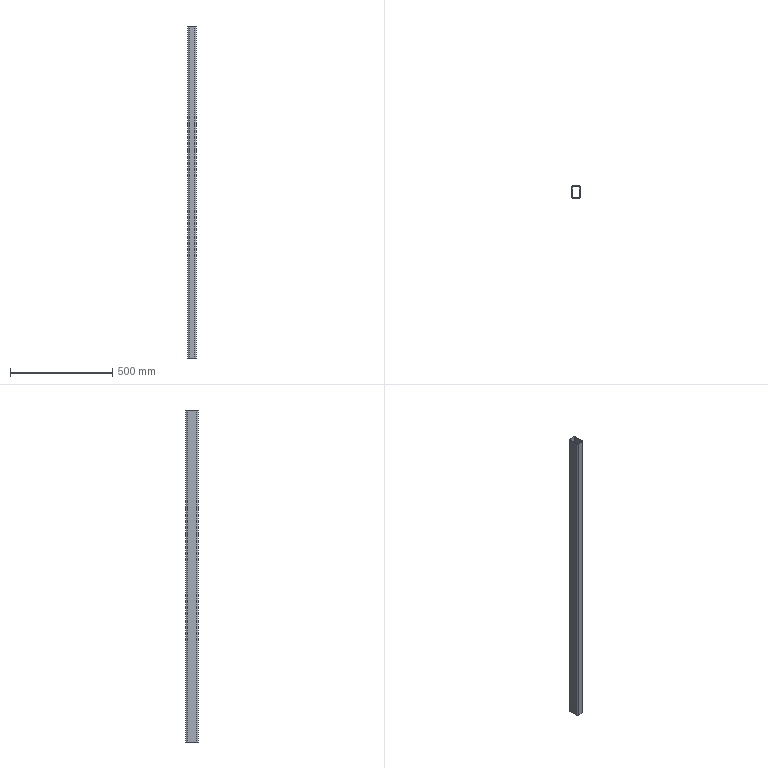Part | STEP file | Profile 40601620 | 1 solid | 18 faces | box 40 x 60 x 1620 mm | volume 927725 mm3 | plane 10 | cylinder 8 | commonest cylinder face diameters 6.4 x4 12.8 x4
STEP:
#1=CARTESIAN_POINT('',(0.,53.6,1020.));
#2=VERTEX_POINT('',#1);
#3=CARTESIAN_POINT('',(0.,6.4,1020.));
#4=VERTEX_POINT('',#3);
#5=CARTESIAN_POINT('',(0.,6.4,1020.));
#6=DIRECTION('',(0.,-1.,0.));
#7=VECTOR('',#6,1000.);
#8=LINE('',#5,#7);
#9=EDGE_CURVE('',#2,#4,#8,.T.);
#10=ORIENTED_EDGE('',*,*,#9,.F.);
#11=CARTESIAN_POINT('',(0.,53.6,-600.));
#12=VERTEX_POINT('',#11);
#13=CARTESIAN_POINT('',(0.,53.6,600.));
#14=DIRECTION('',(0.,0.,1.));
#15=VECTOR('',#14,1000.);
#16=LINE('',#13,#15);
#17=EDGE_CURVE('',#12,#2,#16,.T.);
#18=ORIENTED_EDGE('',*,*,#17,.F.);
#19=CARTESIAN_POINT('',(0.,6.4,-600.));
#20=VERTEX_POINT('',#19);
#21=CARTESIAN_POINT('',(0.,6.4,-600.));
#22=DIRECTION('',(0.,1.,0.));
#23=VECTOR('',#22,1000.);
#24=LINE('',#21,#23);
#25=EDGE_CURVE('',#20,#12,#24,.T.);
#26=ORIENTED_EDGE('',*,*,#25,.F.);
#27=CARTESIAN_POINT('',(0.,6.4,600.));
#28=DIRECTION('',(0.,0.,-1.));
#29=VECTOR('',#28,1000.);
#30=LINE('',#27,#29);
#31=EDGE_CURVE('',#4,#20,#30,.T.);
#32=ORIENTED_EDGE('',*,*,#31,.F.);
#33=EDGE_LOOP('',(#10,#18,#26,#32));
#34=FACE_OUTER_BOUND('',#33,.T.);
#35=CARTESIAN_POINT('',(0.,6.4,600.));
#36=DIRECTION('',(1.,0.,0.));
#37=DIRECTION('',(0.,1.,0.));
#38=AXIS2_PLACEMENT_3D('',#35,#36,#37);
#39=PLANE('',#38);
#40=ADVANCED_FACE('',(#34),#39,.F.);
#41=ORIENTED_EDGE('',*,*,#31,.T.);
#42=CARTESIAN_POINT('',(6.4,0.,-600.));
#43=VERTEX_POINT('',#42);
#44=CARTESIAN_POINT('',(6.4,6.4,-600.));
#45=DIRECTION('',(0.,0.,1.));
#46=DIRECTION('',(-1.,0.,0.));
#47=AXIS2_PLACEMENT_3D('',#44,#45,#46);
#48=CIRCLE('',#47,6.4);
#49=EDGE_CURVE('',#20,#43,#48,.T.);
#50=ORIENTED_EDGE('',*,*,#49,.T.);
#51=CARTESIAN_POINT('',(6.4,0.,1020.));
#52=VERTEX_POINT('',#51);
#53=CARTESIAN_POINT('',(6.4,0.,600.));
#54=DIRECTION('',(0.,0.,1.));
#55=VECTOR('',#54,1000.);
#56=LINE('',#53,#55);
#57=EDGE_CURVE('',#43,#52,#56,.T.);
#58=ORIENTED_EDGE('',*,*,#57,.T.);
#59=CARTESIAN_POINT('',(6.4,6.4,1020.));
#60=DIRECTION('',(0.,0.,-1.));
#61=DIRECTION('',(-1.,0.,0.));
#62=AXIS2_PLACEMENT_3D('',#59,#60,#61);
#63=CIRCLE('',#62,6.4);
#64=EDGE_CURVE('',#52,#4,#63,.T.);
#65=ORIENTED_EDGE('',*,*,#64,.T.);
#66=EDGE_LOOP('',(#41,#50,#58,#65));
#67=FACE_OUTER_BOUND('',#66,.T.);
#68=CARTESIAN_POINT('',(6.4,6.4,600.));
#69=DIRECTION('',(0.,0.,-1.));
#70=DIRECTION('',(-1.,0.,0.));
#71=AXIS2_PLACEMENT_3D('',#68,#69,#70);
#72=CYLINDRICAL_SURFACE('',#71,6.4);
#73=ADVANCED_FACE('',(#67),#72,.T.);
#74=CARTESIAN_POINT('',(6.4,56.8,1020.));
#75=VERTEX_POINT('',#74);
#76=CARTESIAN_POINT('',(33.6,56.8,1020.));
#77=VERTEX_POINT('',#76);
#78=CARTESIAN_POINT('',(33.6,56.8,1020.));
#79=DIRECTION('',(1.,0.,0.));
#80=VECTOR('',#79,1000.);
#81=LINE('',#78,#80);
#82=EDGE_CURVE('',#75,#77,#81,.T.);
#83=ORIENTED_EDGE('',*,*,#82,.T.);
#84=CARTESIAN_POINT('',(36.8,53.6,1020.));
#85=VERTEX_POINT('',#84);
#86=CARTESIAN_POINT('',(33.6,53.6,1020.));
#87=DIRECTION('',(0.,0.,-1.));
#88=DIRECTION('',(-1.,0.,0.));
#89=AXIS2_PLACEMENT_3D('',#86,#87,#88);
#90=CIRCLE('',#89,3.2);
#91=EDGE_CURVE('',#77,#85,#90,.T.);
#92=ORIENTED_EDGE('',*,*,#91,.T.);
#93=CARTESIAN_POINT('',(36.8,6.4,1020.));
#94=VERTEX_POINT('',#93);
#95=CARTESIAN_POINT('',(36.8,6.4,1020.));
#96=DIRECTION('',(0.,-1.,0.));
#97=VECTOR('',#96,1000.);
#98=LINE('',#95,#97);
#99=EDGE_CURVE('',#85,#94,#98,.T.);
#100=ORIENTED_EDGE('',*,*,#99,.T.);
#101=CARTESIAN_POINT('',(33.6,3.2,1020.));
#102=VERTEX_POINT('',#101);
#103=CARTESIAN_POINT('',(33.6,6.4,1020.));
#104=DIRECTION('',(0.,0.,-1.));
#105=DIRECTION('',(-1.,0.,0.));
#106=AXIS2_PLACEMENT_3D('',#103,#104,#105);
#107=CIRCLE('',#106,3.2);
#108=EDGE_CURVE('',#94,#102,#107,.T.);
#109=ORIENTED_EDGE('',*,*,#108,.T.);
#110=CARTESIAN_POINT('',(6.4,3.2,1020.));
#111=VERTEX_POINT('',#110);
#112=CARTESIAN_POINT('',(33.6,3.2,1020.));
#113=DIRECTION('',(-1.,0.,0.));
#114=VECTOR('',#113,1000.);
#115=LINE('',#112,#114);
#116=EDGE_CURVE('',#102,#111,#115,.T.);
#117=ORIENTED_EDGE('',*,*,#116,.T.);
#118=CARTESIAN_POINT('',(3.2,6.4,1020.));
#119=VERTEX_POINT('',#118);
#120=CARTESIAN_POINT('',(6.4,6.4,1020.));
#121=DIRECTION('',(0.,0.,-1.));
#122=DIRECTION('',(-1.,0.,0.));
#123=AXIS2_PLACEMENT_3D('',#120,#121,#122);
#124=CIRCLE('',#123,3.2);
#125=EDGE_CURVE('',#111,#119,#124,.T.);
#126=ORIENTED_EDGE('',*,*,#125,.T.);
#127=CARTESIAN_POINT('',(3.2,53.6,1020.));
#128=VERTEX_POINT('',#127);
#129=CARTESIAN_POINT('',(3.2,6.4,1020.));
#130=DIRECTION('',(0.,1.,0.));
#131=VECTOR('',#130,1000.);
#132=LINE('',#129,#131);
#133=EDGE_CURVE('',#119,#128,#132,.T.);
#134=ORIENTED_EDGE('',*,*,#133,.T.);
#135=CARTESIAN_POINT('',(6.4,53.6,1020.));
#136=DIRECTION('',(0.,0.,-1.));
#137=DIRECTION('',(-1.,0.,0.));
#138=AXIS2_PLACEMENT_3D('',#135,#136,#137);
#139=CIRCLE('',#138,3.2);
#140=EDGE_CURVE('',#128,#75,#139,.T.);
#141=ORIENTED_EDGE('',*,*,#140,.T.);
#142=EDGE_LOOP('',(#83,#92,#100,#109,#117,#126,#134,#141));
#143=FACE_BOUND('',#142,.T.);
#144=ORIENTED_EDGE('',*,*,#64,.F.);
#145=CARTESIAN_POINT('',(33.6,0.,1020.));
#146=VERTEX_POINT('',#145);
#147=CARTESIAN_POINT('',(33.6,0.,1020.));
#148=DIRECTION('',(1.,0.,0.));
#149=VECTOR('',#148,1000.);
#150=LINE('',#147,#149);
#151=EDGE_CURVE('',#52,#146,#150,.T.);
#152=ORIENTED_EDGE('',*,*,#151,.T.);
#153=CARTESIAN_POINT('',(40.,6.4,1020.));
#154=VERTEX_POINT('',#153);
#155=CARTESIAN_POINT('',(33.6,6.4,1020.));
#156=DIRECTION('',(0.,0.,1.));
#157=DIRECTION('',(-1.,0.,0.));
#158=AXIS2_PLACEMENT_3D('',#155,#156,#157);
#159=CIRCLE('',#158,6.4);
#160=EDGE_CURVE('',#146,#154,#159,.T.);
#161=ORIENTED_EDGE('',*,*,#160,.T.);
#162=CARTESIAN_POINT('',(40.,53.6,1020.));
#163=VERTEX_POINT('',#162);
#164=CARTESIAN_POINT('',(40.,6.4,1020.));
#165=DIRECTION('',(0.,1.,0.));
#166=VECTOR('',#165,1000.);
#167=LINE('',#164,#166);
#168=EDGE_CURVE('',#154,#163,#167,.T.);
#169=ORIENTED_EDGE('',*,*,#168,.T.);
#170=CARTESIAN_POINT('',(33.6,60.,1020.));
#171=VERTEX_POINT('',#170);
#172=CARTESIAN_POINT('',(33.6,53.6,1020.));
#173=DIRECTION('',(0.,0.,1.));
#174=DIRECTION('',(-1.,0.,0.));
#175=AXIS2_PLACEMENT_3D('',#172,#173,#174);
#176=CIRCLE('',#175,6.4);
#177=EDGE_CURVE('',#163,#171,#176,.T.);
#178=ORIENTED_EDGE('',*,*,#177,.T.);
#179=CARTESIAN_POINT('',(6.4,60.,1020.));
#180=VERTEX_POINT('',#179);
#181=CARTESIAN_POINT('',(33.6,60.,1020.));
#182=DIRECTION('',(-1.,0.,0.));
#183=VECTOR('',#182,1000.);
#184=LINE('',#181,#183);
#185=EDGE_CURVE('',#171,#180,#184,.T.);
#186=ORIENTED_EDGE('',*,*,#185,.T.);
#187=CARTESIAN_POINT('',(6.4,53.6,1020.));
#188=DIRECTION('',(0.,0.,1.));
#189=DIRECTION('',(-1.,0.,0.));
#190=AXIS2_PLACEMENT_3D('',#187,#188,#189);
#191=CIRCLE('',#190,6.4);
#192=EDGE_CURVE('',#180,#2,#191,.T.);
#193=ORIENTED_EDGE('',*,*,#192,.T.);
#194=ORIENTED_EDGE('',*,*,#9,.T.);
#195=EDGE_LOOP('',(#144,#152,#161,#169,#178,#186,#193,#194));
#196=FACE_OUTER_BOUND('',#195,.T.);
#197=CARTESIAN_POINT('',(33.6,6.4,1020.));
#198=DIRECTION('',(0.,0.,1.));
#199=DIRECTION('',(1.,0.,0.));
#200=AXIS2_PLACEMENT_3D('',#197,#198,#199);
#201=PLANE('',#200);
#202=ADVANCED_FACE('',(#143,#196),#201,.T.);
#203=CARTESIAN_POINT('',(6.4,60.,-600.));
#204=VERTEX_POINT('',#203);
#205=CARTESIAN_POINT('',(6.4,60.,600.));
#206=DIRECTION('',(0.,0.,-1.));
#207=VECTOR('',#206,1000.);
#208=LINE('',#205,#207);
#209=EDGE_CURVE('',#180,#204,#208,.T.);
#210=ORIENTED_EDGE('',*,*,#209,.T.);
#211=CARTESIAN_POINT('',(6.4,53.6,-600.));
#212=DIRECTION('',(0.,0.,1.));
#213=DIRECTION('',(-1.,0.,0.));
#214=AXIS2_PLACEMENT_3D('',#211,#212,#213);
#215=CIRCLE('',#214,6.4);
#216=EDGE_CURVE('',#204,#12,#215,.T.);
#217=ORIENTED_EDGE('',*,*,#216,.T.);
#218=ORIENTED_EDGE('',*,*,#17,.T.);
#219=ORIENTED_EDGE('',*,*,#192,.F.);
#220=EDGE_LOOP('',(#210,#217,#218,#219));
#221=FACE_OUTER_BOUND('',#220,.T.);
#222=CARTESIAN_POINT('',(6.4,53.6,600.));
#223=DIRECTION('',(0.,0.,-1.));
#224=DIRECTION('',(-1.,0.,0.));
#225=AXIS2_PLACEMENT_3D('',#222,#223,#224);
#226=CYLINDRICAL_SURFACE('',#225,6.4);
#227=ADVANCED_FACE('',(#221),#226,.T.);
#228=CARTESIAN_POINT('',(33.6,0.,-600.));
#229=VERTEX_POINT('',#228);
#230=CARTESIAN_POINT('',(40.,6.4,-600.));
#231=VERTEX_POINT('',#230);
#232=CARTESIAN_POINT('',(33.6,6.4,-600.));
#233=DIRECTION('',(0.,0.,1.));
#234=DIRECTION('',(-1.,0.,0.));
#235=AXIS2_PLACEMENT_3D('',#232,#233,#234);
#236=CIRCLE('',#235,6.4);
#237=EDGE_CURVE('',#229,#231,#236,.T.);
#238=ORIENTED_EDGE('',*,*,#237,.F.);
#239=CARTESIAN_POINT('',(33.6,0.,-600.));
#240=DIRECTION('',(1.,0.,0.));
#241=VECTOR('',#240,1000.);
#242=LINE('',#239,#241);
#243=EDGE_CURVE('',#43,#229,#242,.T.);
#244=ORIENTED_EDGE('',*,*,#243,.F.);
#245=ORIENTED_EDGE('',*,*,#49,.F.);
#246=ORIENTED_EDGE('',*,*,#25,.T.);
#247=ORIENTED_EDGE('',*,*,#216,.F.);
#248=CARTESIAN_POINT('',(33.6,60.,-600.));
#249=VERTEX_POINT('',#248);
#250=CARTESIAN_POINT('',(33.6,60.,-600.));
#251=DIRECTION('',(-1.,0.,0.));
#252=VECTOR('',#251,1000.);
#253=LINE('',#250,#252);
#254=EDGE_CURVE('',#249,#204,#253,.T.);
#255=ORIENTED_EDGE('',*,*,#254,.F.);
#256=CARTESIAN_POINT('',(40.,53.6,-600.));
#257=VERTEX_POINT('',#256);
#258=CARTESIAN_POINT('',(33.6,53.6,-600.));
#259=DIRECTION('',(0.,0.,1.));
#260=DIRECTION('',(-1.,0.,0.));
#261=AXIS2_PLACEMENT_3D('',#258,#259,#260);
#262=CIRCLE('',#261,6.4);
#263=EDGE_CURVE('',#257,#249,#262,.T.);
#264=ORIENTED_EDGE('',*,*,#263,.F.);
#265=CARTESIAN_POINT('',(40.,53.6,-600.));
#266=DIRECTION('',(0.,1.,0.));
#267=VECTOR('',#266,1000.);
#268=LINE('',#265,#267);
#269=EDGE_CURVE('',#231,#257,#268,.T.);
#270=ORIENTED_EDGE('',*,*,#269,.F.);
#271=EDGE_LOOP('',(#238,#244,#245,#246,#247,#255,#264,#270));
#272=FACE_OUTER_BOUND('',#271,.T.);
#273=CARTESIAN_POINT('',(6.4,3.2,-600.));
#274=VERTEX_POINT('',#273);
#275=CARTESIAN_POINT('',(3.2,6.4,-600.));
#276=VERTEX_POINT('',#275);
#277=CARTESIAN_POINT('',(6.4,6.4,-600.));
#278=DIRECTION('',(0.,0.,-1.));
#279=DIRECTION('',(-1.,0.,0.));
#280=AXIS2_PLACEMENT_3D('',#277,#278,#279);
#281=CIRCLE('',#280,3.2);
#282=EDGE_CURVE('',#274,#276,#281,.T.);
#283=ORIENTED_EDGE('',*,*,#282,.F.);
#284=CARTESIAN_POINT('',(33.6,3.2,-600.));
#285=VERTEX_POINT('',#284);
#286=CARTESIAN_POINT('',(33.6,3.2,-600.));
#287=DIRECTION('',(-1.,0.,0.));
#288=VECTOR('',#287,1000.);
#289=LINE('',#286,#288);
#290=EDGE_CURVE('',#285,#274,#289,.T.);
#291=ORIENTED_EDGE('',*,*,#290,.F.);
#292=CARTESIAN_POINT('',(36.8,6.4,-600.));
#293=VERTEX_POINT('',#292);
#294=CARTESIAN_POINT('',(33.6,6.4,-600.));
#295=DIRECTION('',(0.,0.,-1.));
#296=DIRECTION('',(-1.,0.,0.));
#297=AXIS2_PLACEMENT_3D('',#294,#295,#296);
#298=CIRCLE('',#297,3.2);
#299=EDGE_CURVE('',#293,#285,#298,.T.);
#300=ORIENTED_EDGE('',*,*,#299,.F.);
#301=CARTESIAN_POINT('',(36.8,53.6,-600.));
#302=VERTEX_POINT('',#301);
#303=CARTESIAN_POINT('',(36.8,53.6,-600.));
#304=DIRECTION('',(0.,-1.,0.));
#305=VECTOR('',#304,1000.);
#306=LINE('',#303,#305);
#307=EDGE_CURVE('',#302,#293,#306,.T.);
#308=ORIENTED_EDGE('',*,*,#307,.F.);
#309=CARTESIAN_POINT('',(33.6,56.8,-600.));
#310=VERTEX_POINT('',#309);
#311=CARTESIAN_POINT('',(33.6,53.6,-600.));
#312=DIRECTION('',(0.,0.,-1.));
#313=DIRECTION('',(-1.,0.,0.));
#314=AXIS2_PLACEMENT_3D('',#311,#312,#313);
#315=CIRCLE('',#314,3.2);
#316=EDGE_CURVE('',#310,#302,#315,.T.);
#317=ORIENTED_EDGE('',*,*,#316,.F.);
#318=CARTESIAN_POINT('',(6.4,56.8,-600.));
#319=VERTEX_POINT('',#318);
#320=CARTESIAN_POINT('',(33.6,56.8,-600.));
#321=DIRECTION('',(1.,0.,0.));
#322=VECTOR('',#321,1000.);
#323=LINE('',#320,#322);
#324=EDGE_CURVE('',#319,#310,#323,.T.);
#325=ORIENTED_EDGE('',*,*,#324,.F.);
#326=CARTESIAN_POINT('',(3.2,53.6,-600.));
#327=VERTEX_POINT('',#326);
#328=CARTESIAN_POINT('',(6.4,53.6,-600.));
#329=DIRECTION('',(0.,0.,-1.));
#330=DIRECTION('',(-1.,0.,0.));
#331=AXIS2_PLACEMENT_3D('',#328,#329,#330);
#332=CIRCLE('',#331,3.2);
#333=EDGE_CURVE('',#327,#319,#332,.T.);
#334=ORIENTED_EDGE('',*,*,#333,.F.);
#335=CARTESIAN_POINT('',(3.2,53.6,-600.));
#336=DIRECTION('',(0.,1.,0.));
#337=VECTOR('',#336,1000.);
#338=LINE('',#335,#337);
#339=EDGE_CURVE('',#276,#327,#338,.T.);
#340=ORIENTED_EDGE('',*,*,#339,.F.);
#341=EDGE_LOOP('',(#283,#291,#300,#308,#317,#325,#334,#340));
#342=FACE_BOUND('',#341,.T.);
#343=CARTESIAN_POINT('',(33.6,53.6,-600.));
#344=DIRECTION('',(0.,0.,1.));
#345=DIRECTION('',(1.,0.,0.));
#346=AXIS2_PLACEMENT_3D('',#343,#344,#345);
#347=PLANE('',#346);
#348=ADVANCED_FACE('',(#272,#342),#347,.F.);
#349=ORIENTED_EDGE('',*,*,#151,.F.);
#350=ORIENTED_EDGE('',*,*,#57,.F.);
#351=ORIENTED_EDGE('',*,*,#243,.T.);
#352=CARTESIAN_POINT('',(33.6,0.,600.));
#353=DIRECTION('',(0.,0.,-1.));
#354=VECTOR('',#353,1000.);
#355=LINE('',#352,#354);
#356=EDGE_CURVE('',#146,#229,#355,.T.);
#357=ORIENTED_EDGE('',*,*,#356,.F.);
#358=EDGE_LOOP('',(#349,#350,#351,#357));
#359=FACE_OUTER_BOUND('',#358,.T.);
#360=CARTESIAN_POINT('',(6.4,0.,600.));
#361=DIRECTION('',(0.,1.,0.));
#362=DIRECTION('',(-1.,0.,0.));
#363=AXIS2_PLACEMENT_3D('',#360,#361,#362);
#364=PLANE('',#363);
#365=ADVANCED_FACE('',(#359),#364,.F.);
#366=ORIENTED_EDGE('',*,*,#91,.F.);
#367=CARTESIAN_POINT('',(33.6,56.8,600.));
#368=DIRECTION('',(0.,0.,1.));
#369=VECTOR('',#368,1000.);
#370=LINE('',#367,#369);
#371=EDGE_CURVE('',#310,#77,#370,.T.);
#372=ORIENTED_EDGE('',*,*,#371,.F.);
#373=ORIENTED_EDGE('',*,*,#316,.T.);
#374=CARTESIAN_POINT('',(36.8,53.6,600.));
#375=DIRECTION('',(0.,0.,-1.));
#376=VECTOR('',#375,1000.);
#377=LINE('',#374,#376);
#378=EDGE_CURVE('',#85,#302,#377,.T.);
#379=ORIENTED_EDGE('',*,*,#378,.F.);
#380=EDGE_LOOP('',(#366,#372,#373,#379));
#381=FACE_OUTER_BOUND('',#380,.T.);
#382=CARTESIAN_POINT('',(33.6,53.6,600.));
#383=DIRECTION('',(0.,0.,-1.));
#384=DIRECTION('',(-1.,0.,0.));
#385=AXIS2_PLACEMENT_3D('',#382,#383,#384);
#386=CYLINDRICAL_SURFACE('',#385,3.2);
#387=ADVANCED_FACE('',(#381),#386,.F.);
#388=CARTESIAN_POINT('',(6.4,56.8,600.));
#389=DIRECTION('',(0.,0.,-1.));
#390=VECTOR('',#389,1000.);
#391=LINE('',#388,#390);
#392=EDGE_CURVE('',#75,#319,#391,.T.);
#393=ORIENTED_EDGE('',*,*,#392,.T.);
#394=ORIENTED_EDGE('',*,*,#324,.T.);
#395=ORIENTED_EDGE('',*,*,#371,.T.);
#396=ORIENTED_EDGE('',*,*,#82,.F.);
#397=EDGE_LOOP('',(#393,#394,#395,#396));
#398=FACE_OUTER_BOUND('',#397,.T.);
#399=CARTESIAN_POINT('',(33.6,56.8,600.));
#400=DIRECTION('',(0.,-1.,0.));
#401=DIRECTION('',(0.,0.,-1.));
#402=AXIS2_PLACEMENT_3D('',#399,#400,#401);
#403=PLANE('',#402);
#404=ADVANCED_FACE('',(#398),#403,.T.);
#405=ORIENTED_EDGE('',*,*,#140,.F.);
#406=CARTESIAN_POINT('',(3.2,53.6,600.));
#407=DIRECTION('',(0.,0.,1.));
#408=VECTOR('',#407,1000.);
#409=LINE('',#406,#408);
#410=EDGE_CURVE('',#327,#128,#409,.T.);
#411=ORIENTED_EDGE('',*,*,#410,.F.);
#412=ORIENTED_EDGE('',*,*,#333,.T.);
#413=ORIENTED_EDGE('',*,*,#392,.F.);
#414=EDGE_LOOP('',(#405,#411,#412,#413));
#415=FACE_OUTER_BOUND('',#414,.T.);
#416=CARTESIAN_POINT('',(6.4,53.6,600.));
#417=DIRECTION('',(0.,0.,-1.));
#418=DIRECTION('',(-1.,0.,0.));
#419=AXIS2_PLACEMENT_3D('',#416,#417,#418);
#420=CYLINDRICAL_SURFACE('',#419,3.2);
#421=ADVANCED_FACE('',(#415),#420,.F.);
#422=CARTESIAN_POINT('',(3.2,6.4,600.));
#423=DIRECTION('',(0.,0.,-1.));
#424=VECTOR('',#423,1000.);
#425=LINE('',#422,#424);
#426=EDGE_CURVE('',#119,#276,#425,.T.);
#427=ORIENTED_EDGE('',*,*,#426,.T.);
#428=ORIENTED_EDGE('',*,*,#339,.T.);
#429=ORIENTED_EDGE('',*,*,#410,.T.);
#430=ORIENTED_EDGE('',*,*,#133,.F.);
#431=EDGE_LOOP('',(#427,#428,#429,#430));
#432=FACE_OUTER_BOUND('',#431,.T.);
#433=CARTESIAN_POINT('',(3.2,6.4,600.));
#434=DIRECTION('',(1.,0.,0.));
#435=DIRECTION('',(0.,1.,0.));
#436=AXIS2_PLACEMENT_3D('',#433,#434,#435);
#437=PLANE('',#436);
#438=ADVANCED_FACE('',(#432),#437,.T.);
#439=ORIENTED_EDGE('',*,*,#125,.F.);
#440=CARTESIAN_POINT('',(6.4,3.2,600.));
#441=DIRECTION('',(0.,0.,1.));
#442=VECTOR('',#441,1000.);
#443=LINE('',#440,#442);
#444=EDGE_CURVE('',#274,#111,#443,.T.);
#445=ORIENTED_EDGE('',*,*,#444,.F.);
#446=ORIENTED_EDGE('',*,*,#282,.T.);
#447=ORIENTED_EDGE('',*,*,#426,.F.);
#448=EDGE_LOOP('',(#439,#445,#446,#447));
#449=FACE_OUTER_BOUND('',#448,.T.);
#450=CARTESIAN_POINT('',(6.4,6.4,600.));
#451=DIRECTION('',(0.,0.,-1.));
#452=DIRECTION('',(-1.,0.,0.));
#453=AXIS2_PLACEMENT_3D('',#450,#451,#452);
#454=CYLINDRICAL_SURFACE('',#453,3.2);
#455=ADVANCED_FACE('',(#449),#454,.F.);
#456=CARTESIAN_POINT('',(33.6,3.2,600.));
#457=DIRECTION('',(0.,0.,-1.));
#458=VECTOR('',#457,1000.);
#459=LINE('',#456,#458);
#460=EDGE_CURVE('',#102,#285,#459,.T.);
#461=ORIENTED_EDGE('',*,*,#460,.T.);
#462=ORIENTED_EDGE('',*,*,#290,.T.);
#463=ORIENTED_EDGE('',*,*,#444,.T.);
#464=ORIENTED_EDGE('',*,*,#116,.F.);
#465=EDGE_LOOP('',(#461,#462,#463,#464));
#466=FACE_OUTER_BOUND('',#465,.T.);
#467=CARTESIAN_POINT('',(6.4,3.2,600.));
#468=DIRECTION('',(0.,1.,0.));
#469=DIRECTION('',(-1.,0.,0.));
#470=AXIS2_PLACEMENT_3D('',#467,#468,#469);
#471=PLANE('',#470);
#472=ADVANCED_FACE('',(#466),#471,.T.);
#473=ORIENTED_EDGE('',*,*,#108,.F.);
#474=CARTESIAN_POINT('',(36.8,6.4,600.));
#475=DIRECTION('',(0.,0.,1.));
#476=VECTOR('',#475,1000.);
#477=LINE('',#474,#476);
#478=EDGE_CURVE('',#293,#94,#477,.T.);
#479=ORIENTED_EDGE('',*,*,#478,.F.);
#480=ORIENTED_EDGE('',*,*,#299,.T.);
#481=ORIENTED_EDGE('',*,*,#460,.F.);
#482=EDGE_LOOP('',(#473,#479,#480,#481));
#483=FACE_OUTER_BOUND('',#482,.T.);
#484=CARTESIAN_POINT('',(33.6,6.4,600.));
#485=DIRECTION('',(0.,0.,-1.));
#486=DIRECTION('',(-1.,0.,0.));
#487=AXIS2_PLACEMENT_3D('',#484,#485,#486);
#488=CYLINDRICAL_SURFACE('',#487,3.2);
#489=ADVANCED_FACE('',(#483),#488,.F.);
#490=ORIENTED_EDGE('',*,*,#378,.T.);
#491=ORIENTED_EDGE('',*,*,#307,.T.);
#492=ORIENTED_EDGE('',*,*,#478,.T.);
#493=ORIENTED_EDGE('',*,*,#99,.F.);
#494=EDGE_LOOP('',(#490,#491,#492,#493));
#495=FACE_OUTER_BOUND('',#494,.T.);
#496=CARTESIAN_POINT('',(36.8,53.6,600.));
#497=DIRECTION('',(-1.,0.,0.));
#498=DIRECTION('',(0.,0.,1.));
#499=AXIS2_PLACEMENT_3D('',#496,#497,#498);
#500=PLANE('',#499);
#501=ADVANCED_FACE('',(#495),#500,.T.);
#502=ORIENTED_EDGE('',*,*,#185,.F.);
#503=CARTESIAN_POINT('',(33.6,60.,600.));
#504=DIRECTION('',(0.,0.,1.));
#505=VECTOR('',#504,1000.);
#506=LINE('',#503,#505);
#507=EDGE_CURVE('',#249,#171,#506,.T.);
#508=ORIENTED_EDGE('',*,*,#507,.F.);
#509=ORIENTED_EDGE('',*,*,#254,.T.);
#510=ORIENTED_EDGE('',*,*,#209,.F.);
#511=EDGE_LOOP('',(#502,#508,#509,#510));
#512=FACE_OUTER_BOUND('',#511,.T.);
#513=CARTESIAN_POINT('',(33.6,60.,600.));
#514=DIRECTION('',(0.,-1.,0.));
#515=DIRECTION('',(0.,0.,-1.));
#516=AXIS2_PLACEMENT_3D('',#513,#514,#515);
#517=PLANE('',#516);
#518=ADVANCED_FACE('',(#512),#517,.F.);
#519=CARTESIAN_POINT('',(40.,53.6,600.));
#520=DIRECTION('',(0.,0.,-1.));
#521=VECTOR('',#520,1000.);
#522=LINE('',#519,#521);
#523=EDGE_CURVE('',#163,#257,#522,.T.);
#524=ORIENTED_EDGE('',*,*,#523,.T.);
#525=ORIENTED_EDGE('',*,*,#263,.T.);
#526=ORIENTED_EDGE('',*,*,#507,.T.);
#527=ORIENTED_EDGE('',*,*,#177,.F.);
#528=EDGE_LOOP('',(#524,#525,#526,#527));
#529=FACE_OUTER_BOUND('',#528,.T.);
#530=CARTESIAN_POINT('',(33.6,53.6,600.));
#531=DIRECTION('',(0.,0.,-1.));
#532=DIRECTION('',(-1.,0.,0.));
#533=AXIS2_PLACEMENT_3D('',#530,#531,#532);
#534=CYLINDRICAL_SURFACE('',#533,6.4);
#535=ADVANCED_FACE('',(#529),#534,.T.);
#536=ORIENTED_EDGE('',*,*,#168,.F.);
#537=CARTESIAN_POINT('',(40.,6.4,600.));
#538=DIRECTION('',(0.,0.,1.));
#539=VECTOR('',#538,1000.);
#540=LINE('',#537,#539);
#541=EDGE_CURVE('',#231,#154,#540,.T.);
#542=ORIENTED_EDGE('',*,*,#541,.F.);
#543=ORIENTED_EDGE('',*,*,#269,.T.);
#544=ORIENTED_EDGE('',*,*,#523,.F.);
#545=EDGE_LOOP('',(#536,#542,#543,#544));
#546=FACE_OUTER_BOUND('',#545,.T.);
#547=CARTESIAN_POINT('',(40.,53.6,600.));
#548=DIRECTION('',(-1.,0.,0.));
#549=DIRECTION('',(0.,0.,1.));
#550=AXIS2_PLACEMENT_3D('',#547,#548,#549);
#551=PLANE('',#550);
#552=ADVANCED_FACE('',(#546),#551,.F.);
#553=ORIENTED_EDGE('',*,*,#356,.T.);
#554=ORIENTED_EDGE('',*,*,#237,.T.);
#555=ORIENTED_EDGE('',*,*,#541,.T.);
#556=ORIENTED_EDGE('',*,*,#160,.F.);
#557=EDGE_LOOP('',(#553,#554,#555,#556));
#558=FACE_OUTER_BOUND('',#557,.T.);
#559=CARTESIAN_POINT('',(33.6,6.4,600.));
#560=DIRECTION('',(0.,0.,-1.));
#561=DIRECTION('',(-1.,0.,0.));
#562=AXIS2_PLACEMENT_3D('',#559,#560,#561);
#563=CYLINDRICAL_SURFACE('',#562,6.4);
#564=ADVANCED_FACE('',(#558),#563,.T.);
#565=CLOSED_SHELL('',(#40,#73,#202,#227,#348,#365,#387,#404,#421,#438,#455,#472,#489,#501,#518,#535,#552,#564));
#566=MANIFOLD_SOLID_BREP('',#565);
#567=CARTESIAN_POINT('',(0.,0.,0.));
#568=DIRECTION('',(0.,0.,1.));
#569=DIRECTION('',(1.,0.,0.));
#570=AXIS2_PLACEMENT_3D('',#567,#568,#569);
#571=(LENGTH_UNIT()NAMED_UNIT(*)SI_UNIT(.MILLI.,.METRE.));
#572=UNCERTAINTY_MEASURE_WITH_UNIT(LENGTH_MEASURE(0.00001),#571,'','');
#573=(NAMED_UNIT(*)PLANE_ANGLE_UNIT()SI_UNIT($,.RADIAN.));
#574=(NAMED_UNIT(*)SI_UNIT($,.STERADIAN.)SOLID_ANGLE_UNIT());
#575=(GEOMETRIC_REPRESENTATION_CONTEXT(3)GLOBAL_UNCERTAINTY_ASSIGNED_CONTEXT((#572))GLOBAL_UNIT_ASSIGNED_CONTEXT((#571,#573,#574))REPRESENTATION_CONTEXT('',''));
#576=ADVANCED_BREP_SHAPE_REPRESENTATION('',(#566,#570),#575);